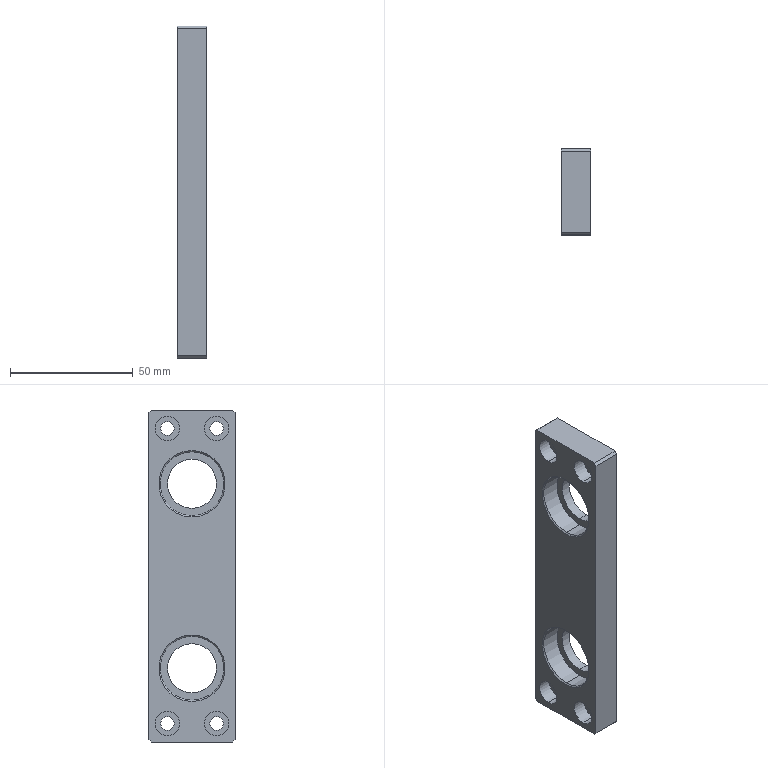Part | STEP file | Bearing support plate | 1 solid | 44 faces | box 12 x 35 x 135 mm | volume 43258 mm3 | cylinder 24 | plane 16 | cone 4 | commonest cylinder face diameters 5.5 x8 10 x8 20 x4 26 x4